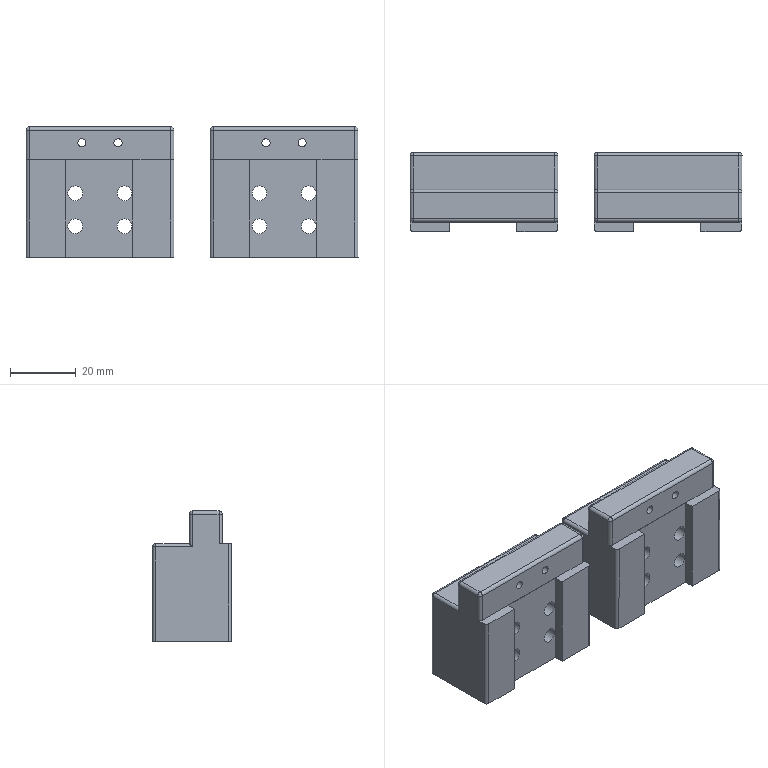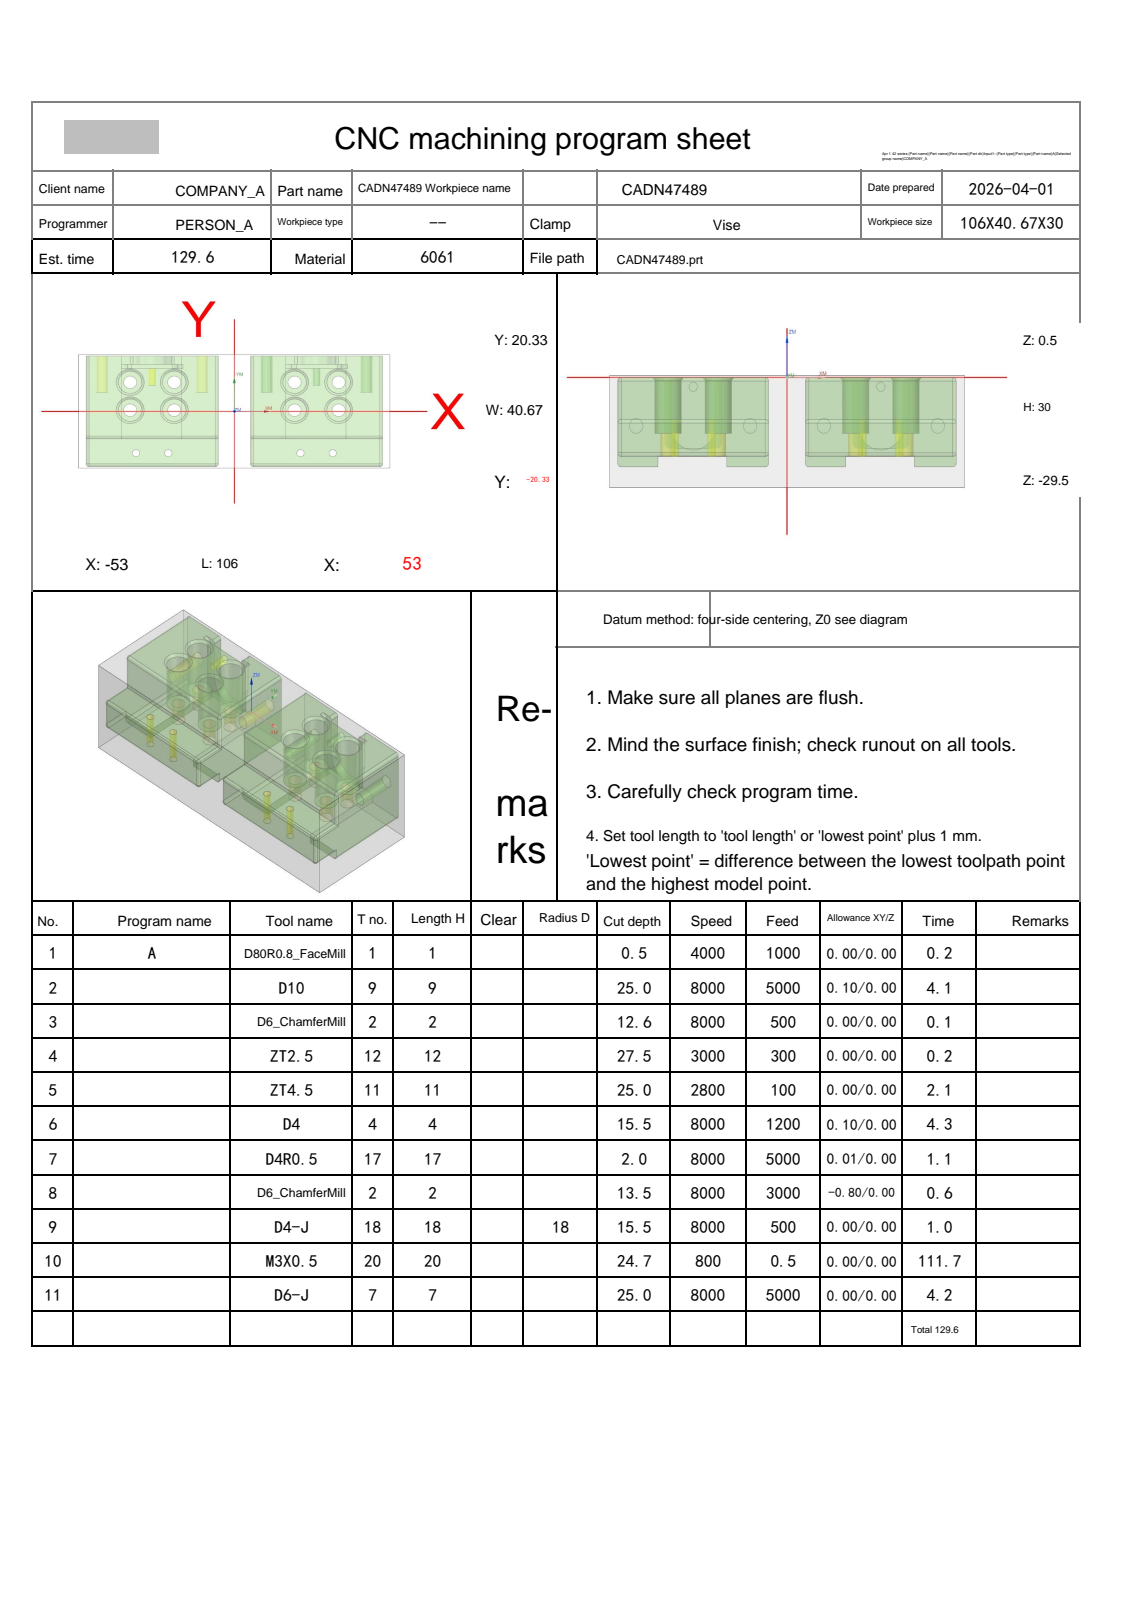NC program | NX | posted by the shop | part box 101.001 x 24.001 x 39.667 mm
Lines 2474 to 3550 of 28944:
N6 T04 M06
(D4  D=4. R=0. H=04 ce=0.10 di=0.00)
G00 G90 G54 X35.5 Y.416 M03 S8000
G43 H04 Z20.
M08
Z.499
G01 X35.513 Y.251 F1200.
X35.555 Y.091
X35.626 Y-.06
X35.721 Y-.196
X35.838 Y-.313
X35.974 Y-.408
X36.124 Y-.478
X36.285 Y-.521
X36.45 Y-.536
X36.615 Y-.521
X36.776 Y-.478
X36.926 Y-.408
X37.062 Y-.313
X37.179 Y-.196
X37.275 Y-.06
X37.345 Y.091
X37.388 Y.251
X37.4 Y.416
X37.386 Y.662 Z.493
X37.338 Y.904 Z.487
X37.26 Y1.138 Z.48
X37.152 Y1.359 Z.474
X37.016 Y1.565 Z.468
X36.855 Y1.752 Z.462
X36.671 Y1.916 Z.456
X36.467 Y2.054 Z.449
X36.247 Y2.166 Z.443
X36.014 Y2.248 Z.437
X35.773 Y2.299 Z.431
X35.528 Y2.318 Z.425
X35.281 Y2.306 Z.419
X35.039 Y2.262 Z.412
X34.804 Y2.186 Z.406
X34.581 Y2.082 Z.4
X34.373 Y1.949 Z.394
X34.185 Y1.79 Z.388
X34.018 Y1.608 Z.381
X33.876 Y1.407 Z.375
X33.762 Y1.188 Z.369
X33.677 Y.957 Z.363
X33.622 Y.717 Z.357
X33.599 Y.471 Z.35
X33.608 Y.225 Z.344
X33.648 Y-.018 Z.338
X33.72 Y-.254 Z.332
X33.822 Y-.479 Z.326
X33.952 Y-.688 Z.319
X34.107 Y-.879 Z.313
X34.287 Y-1.048 Z.307
X34.486 Y-1.193 Z.301
X34.703 Y-1.311 Z.295
X34.933 Y-1.399 Z.288
X35.173 Y-1.457 Z.282
X35.418 Y-1.484 Z.276
X35.664 Y-1.479 Z.27
X35.908 Y-1.441 Z.264
X36.145 Y-1.373 Z.257
X36.371 Y-1.275 Z.251
X36.582 Y-1.148 Z.245
X36.775 Y-.995 Z.239
X36.947 Y-.818 Z.233
X37.095 Y-.62 Z.226
X37.215 Y-.405 Z.22
X37.307 Y-.177 Z.214
X37.369 Y.062 Z.208
X37.399 Y.307 Z.202
X37.397 Y.553 Z.196
X37.364 Y.797 Z.189
X37.299 Y1.035 Z.183
X37.203 Y1.263 Z.177
X37.08 Y1.476 Z.171
X36.929 Y1.671 Z.165
X36.755 Y1.845 Z.158
X36.56 Y1.996 Z.152
X36.347 Y2.12 Z.146
X36.119 Y2.215 Z.14
X35.881 Y2.28 Z.134
X35.637 Y2.313 Z.127
X35.391 Y2.315 Z.121
X35.146 Y2.285 Z.115
X34.907 Y2.224 Z.109
X34.679 Y2.132 Z.103
X34.464 Y2.011 Z.097
X34.266 Y1.864 Z.09
X34.089 Y1.692 Z.084
X33.936 Y1.499 Z.078
X33.809 Y1.287 Z.072
X33.711 Y1.061 Z.066
X33.642 Y.825 Z.059
X33.605 Y.581 Z.053
X33.6 Y.334 Z.047
X33.626 Y.089 Z.041
X33.684 Y-.15 Z.035
X33.773 Y-.38 Z.028
X33.89 Y-.597 Z.022
X34.035 Y-.797 Z.016
X34.204 Y-.976 Z.01
X34.395 Y-1.132 Z.004
X34.605 Y-1.262 Z-.003
X34.829 Y-1.363 Z-.009
X35.065 Y-1.435 Z-.015
X35.308 Y-1.476 Z-.021
X35.555 Y-1.485 Z-.027
X35.8 Y-1.462 Z-.034
X36.04 Y-1.407 Z-.04
X36.272 Y-1.322 Z-.046
X36.49 Y-1.208 Z-.052
X36.692 Y-1.066 Z-.058
X36.873 Y-.899 Z-.065
X37.032 Y-.711 Z-.071
X37.165 Y-.503 Z-.077
X37.27 Y-.28 Z-.083
X37.345 Y-.045 Z-.089
X37.389 Y.197 Z-.096
X37.402 Y.443 Z-.102
X37.382 Y.689 Z-.108
X37.331 Y.93 Z-.114
X37.249 Y1.163 Z-.12
X37.138 Y1.383 Z-.126
X36.999 Y1.587 Z-.133
X36.836 Y1.771 Z-.139
X36.649 Y1.932 Z-.145
X36.443 Y2.068 Z-.151
X36.222 Y2.176 Z-.157
X35.988 Y2.255 Z-.164
X35.746 Y2.302 Z-.17
X35.5 Y2.318 Z-.176
X35.254 Y2.302 Z-.182
X35.013 Y2.255 Z-.188
X34.779 Y2.176 Z-.195
X34.557 Y2.068 Z-.201
X34.352 Y1.933 Z-.207
X34.165 Y1.771 Z-.213
X34.001 Y1.587 Z-.219
X33.862 Y1.384 Z-.226
X33.751 Y1.164 Z-.232
X33.669 Y.931 Z-.238
X33.618 Y.69 Z-.244
X33.598 Y.444 Z-.25
X33.611 Y.198 Z-.257
X33.655 Y-.044 Z-.263
X33.73 Y-.279 Z-.269
X33.835 Y-.502 Z-.275
X33.967 Y-.71 Z-.281
X34.126 Y-.899 Z-.288
X34.308 Y-1.065 Z-.294
X34.509 Y-1.207 Z-.3
X34.728 Y-1.322 Z-.306
X34.959 Y-1.407 Z-.312
X35.199 Y-1.462 Z-.319
X35.445 Y-1.485 Z-.325
X35.691 Y-1.476 Z-.331
X35.934 Y-1.435 Z-.337
X36.17 Y-1.364 Z-.343
X36.395 Y-1.262 Z-.349
X36.604 Y-1.132 Z-.356
X36.795 Y-.976 Z-.362
X36.965 Y-.797 Z-.368
X37.109 Y-.598 Z-.374
X37.227 Y-.381 Z-.38
X37.315 Y-.151 Z-.387
X37.374 Y.089 Z-.393
X37.4 Y.334 Z-.399
X37.395 Y.58 Z-.405
X37.358 Y.824 Z-.411
X37.29 Y1.061 Z-.418
X37.191 Y1.287 Z-.424
X37.064 Y1.498 Z-.43
X36.911 Y1.691 Z-.436
X36.735 Y1.863 Z-.442
X36.537 Y2.011 Z-.448
X36.322 Y2.131 Z-.455
X36.094 Y2.223 Z-.461
X35.855 Y2.285 Z-.467
X35.61 Y2.315 Z-.473
X35.364 Y2.314 Z-.479
X35.119 Y2.28 Z-.486
X34.882 Y2.215 Z-.492
X34.654 Y2.12 Z-.498
X34.441 Y1.996 Z-.504
X34.246 Y1.846 Z-.51
X34.071 Y1.672 Z-.517
X33.921 Y1.476 Z-.523
X33.797 Y1.263 Z-.529
X33.702 Y1.036 Z-.535
X33.637 Y.798 Z-.541
X33.603 Y.554 Z-.548
X33.601 Y.307 Z-.554
X33.631 Y.063 Z-.56
X33.693 Y-.176 Z-.566
X33.784 Y-.405 Z-.572
X33.905 Y-.62 Z-.579
X34.052 Y-.817 Z-.585
X34.224 Y-.994 Z-.591
X34.417 Y-1.147 Z-.597
X34.629 Y-1.274 Z-.603
X34.855 Y-1.373 Z-.61
X35.091 Y-1.441 Z-.616
X35.335 Y-1.478 Z-.622
X35.582 Y-1.484 Z-.628
X35.827 Y-1.457 Z-.634
X36.066 Y-1.399 Z-.641
X36.296 Y-1.311 Z-.647
X36.513 Y-1.193 Z-.653
X36.713 Y-1.049 Z-.659
X36.892 Y-.88 Z-.665
X37.048 Y-.689 Z-.671
X37.178 Y-.479 Z-.678
X37.28 Y-.255 Z-.684
X37.352 Y-.019 Z-.69
X37.392 Y.224 Z-.696
X37.401 Y.471 Z-.702
X37.378 Y.716 Z-.709
X37.324 Y.956 Z-.715
X37.239 Y1.188 Z-.721
X37.124 Y1.406 Z-.727
X36.983 Y1.608 Z-.733
X36.816 Y1.79 Z-.739
X36.627 Y1.948 Z-.746
X36.42 Y2.081 Z-.752
X36.197 Y2.186 Z-.758
X35.962 Y2.261 Z-.764
X35.72 Y2.306 Z-.77
X35.473 Y2.318 Z-.777
X35.228 Y2.299 Z-.783
X34.986 Y2.248 Z-.789
X34.754 Y2.166 Z-.795
X34.534 Y2.055 Z-.801
X34.33 Y1.916 Z-.808
X34.146 Y1.752 Z-.814
X33.985 Y1.566 Z-.82
X33.849 Y1.36 Z-.826
X33.741 Y1.139 Z-.832
X33.662 Y.905 Z-.839
X33.614 Y.663 Z-.845
X33.598 Y.417 Z-.851
X33.614 Y.171 Z-.857
X33.661 Y-.071 Z-.863
X33.74 Y-.304 Z-.87
X33.848 Y-.526 Z-.876
X33.984 Y-.732 Z-.882
X34.145 Y-.918 Z-.888
X34.329 Y-1.082 Z-.894
X34.533 Y-1.221 Z-.901
X34.752 Y-1.333 Z-.907
X34.985 Y-1.415 Z-.913
X35.226 Y-1.466 Z-.919
X35.472 Y-1.485 Z-.925
X35.718 Y-1.473 Z-.932
X35.961 Y-1.429 Z-.938
X36.195 Y-1.354 Z-.944
X36.418 Y-1.249 Z-.95
X36.626 Y-1.116 Z-.956
X36.815 Y-.958 Z-.963
X36.982 Y-.776 Z-.969
X37.123 Y-.575 Z-.975
X37.238 Y-.356 Z-.981
X37.323 Y-.125 Z-.987
X37.378 Y.115 Z-.993
X37.401 Y.361 Z-1.
X37.392 Y.607 Z-1.006
X37.352 Y.85 Z-1.012
X37.28 Y1.086 Z-1.018
X37.179 Y1.311 Z-1.024
X37.049 Y1.52 Z-1.031
X36.893 Y1.711 Z-1.037
X36.714 Y1.881 Z-1.043
X36.514 Y2.025 Z-1.049
X36.298 Y2.143 Z-1.055
X36.068 Y2.232 Z-1.061
X35.828 Y2.29 Z-1.068
X35.583 Y2.317 Z-1.074
X35.337 Y2.311 Z-1.08
X35.093 Y2.274 Z-1.086
X34.856 Y2.206 Z-1.092
X34.63 Y2.108 Z-1.099
X34.419 Y1.981 Z-1.105
X34.225 Y1.828 Z-1.111
X34.053 Y1.651 Z-1.117
X33.906 Y1.454 Z-1.123
X33.785 Y1.239 Z-1.13
X33.693 Y1.01 Z-1.136
X33.632 Y.772 Z-1.142
X33.601 Y.527 Z-1.148
X33.603 Y.28 Z-1.154
X33.636 Y.036 Z-1.161
X33.701 Y-.202 Z-1.167
X33.796 Y-.429 Z-1.173
X33.92 Y-.642 Z-1.179
X34.07 Y-.838 Z-1.185
X34.244 Y-1.012 Z-1.192
X34.44 Y-1.163 Z-1.198
X34.653 Y-1.286 Z-1.204
X34.88 Y-1.382 Z-1.21
X35.118 Y-1.447 Z-1.216
X35.362 Y-1.481 Z-1.223
X35.609 Y-1.482 Z-1.229
X35.853 Y-1.452 Z-1.235
X36.092 Y-1.391 Z-1.241
X36.321 Y-1.299 Z-1.247
X36.536 Y-1.179 Z-1.254
X36.733 Y-1.031 Z-1.26
X36.91 Y-.86 Z-1.266
X37.064 Y-.667 Z-1.272
X37.191 Y-.455 Z-1.278
X37.289 Y-.229 Z-1.285
X37.358 Y.007 Z-1.291
X37.395 Y.251 Z-1.297
X37.4 Y.498 Z-1.303
X37.374 Y.743 Z-1.309
X37.316 Y.982 Z-1.315
X37.227 Y1.212 Z-1.322
X37.11 Y1.429 Z-1.328
X36.966 Y1.629 Z-1.334
X36.796 Y1.808 Z-1.34
X36.606 Y1.964 Z-1.346
X36.396 Y2.094 Z-1.353
X36.172 Y2.196 Z-1.359
X35.936 Y2.268 Z-1.365
X35.693 Y2.309 Z-1.371
X35.446 Y2.318 Z-1.377
X35.201 Y2.295 Z-1.383
X34.96 Y2.24 Z-1.39
X34.729 Y2.155 Z-1.396
X34.511 Y2.041 Z-1.402
X34.309 Y1.899 Z-1.408
X34.127 Y1.733 Z-1.414
X33.968 Y1.544 Z-1.421
X33.835 Y1.337 Z-1.427
X33.73 Y1.114 Z-1.433
X33.655 Y.879 Z-1.439
X33.611 Y.636 Z-1.445
X33.598 Y.39 Z-1.452
X33.618 Y.144 Z-1.458
X33.669 Y-.097 Z-1.464
X33.75 Y-.329 Z-1.47
X33.861 Y-.549 Z-1.476
X34. Y-.753 Z-1.483
X34.164 Y-.937 Z-1.489
X34.35 Y-1.099 Z-1.495
X34.556 Y-1.235 Z-1.501
X34.777 Y-1.343 Z-1.507
X35.011 Y-1.422 Z-1.514
X35.253 Y-1.469 Z-1.52
X35.499 Y-1.486 Z-1.526
X35.745 Y-1.47 Z-1.532
X35.987 Y-1.422 Z-1.538
X36.22 Y-1.344 Z-1.545
X36.442 Y-1.236 Z-1.551
X36.648 Y-1.1 Z-1.557
X36.834 Y-.939 Z-1.563
X36.998 Y-.755 Z-1.569
X37.137 Y-.551 Z-1.576
X37.249 Y-.332 Z-1.582
X37.331 Y-.099 Z-1.588
X37.382 Y.142 Z-1.594
X37.402 Y.388 Z-1.6
X37.39 Y.634 Z-1.606
X37.346 Y.877 Z-1.613
X37.271 Y1.111 Z-1.619
X37.166 Y1.335 Z-1.625
X37.033 Y1.542 Z-1.631
X36.875 Y1.731 Z-1.637
X36.693 Y1.898 Z-1.644
X36.491 Y2.04 Z-1.65
X36.273 Y2.154 Z-1.656
X36.042 Y2.24 Z-1.662
X35.802 Y2.294 Z-1.668
X35.556 Y2.318 Z-1.675
X35.31 Y2.309 Z-1.681
X35.067 Y2.268 Z-1.687
X34.831 Y2.197 Z-1.693
X34.606 Y2.095 Z-1.699
X34.396 Y1.966 Z-1.706
X34.205 Y1.81 Z-1.712
X34.036 Y1.631 Z-1.718
X33.891 Y1.431 Z-1.724
X33.774 Y1.215 Z-1.73
X33.685 Y.985 Z-1.737
X33.627 Y.745 Z-1.743
X33.6 Y.5 Z-1.749
X33.605 Y.254 Z-1.755
X33.642 Y.01 Z-1.761
X33.71 Y-.227 Z-1.768
X33.808 Y-.453 Z-1.774
X33.935 Y-.665 Z-1.78
X34.088 Y-.858 Z-1.786
X34.265 Y-1.03 Z-1.792
X34.462 Y-1.177 Z-1.799
X34.677 Y-1.298 Z-1.805
X34.906 Y-1.39 Z-1.811
X35.144 Y-1.452 Z-1.817
X35.389 Y-1.482 Z-1.823
X35.636 Y-1.481 Z-1.829
X35.88 Y-1.447 Z-1.836
X36.118 Y-1.382 Z-1.842
X36.345 Y-1.287 Z-1.848
X36.558 Y-1.164 Z-1.854
X36.754 Y-1.014 Z-1.86
X36.928 Y-.84 Z-1.867
X37.079 Y-.644 Z-1.873
X37.203 Y-.431 Z-1.879
X37.298 Y-.204 Z-1.885
X37.363 Y.034 Z-1.891
X37.397 Y.278 Z-1.898
X37.399 Y.525 Z-1.904
X37.369 Y.769 Z-1.91
X37.308 Y1.008 Z-1.916
X37.216 Y1.237 Z-1.922
X37.095 Y1.452 Z-1.928
X36.948 Y1.65 Z-1.935
X36.777 Y1.826 Z-1.941
X36.583 Y1.98 Z-1.947
X36.372 Y2.107 Z-1.953
X36.146 Y2.205 Z-1.959
X35.909 Y2.274 Z-1.966
X35.666 Y2.311 Z-1.972
X35.419 Y2.317 Z-1.978
X35.174 Y2.29 Z-1.984
X34.935 Y2.232 Z-1.99
X34.704 Y2.144 Z-1.997
X34.488 Y2.027 Z-2.003
X34.288 Y1.882 Z-2.009
X34.109 Y1.713 Z-2.015
X33.953 Y1.522 Z-2.021
X33.823 Y1.313 Z-2.028
X33.721 Y1.088 Z-2.034
X33.649 Y.853 Z-2.04
X33.608 Y.609 Z-2.046
X33.599 Y.363 Z-2.052
X33.622 Y.118 Z-2.059
X33.676 Y-.123 Z-2.065
X33.761 Y-.354 Z-2.071
X33.875 Y-.573 Z-2.077
X34.017 Y-.774 Z-2.083
X34.183 Y-.956 Z-2.09
X34.372 Y-1.115 Z-2.096
X34.58 Y-1.248 Z-2.102
X34.803 Y-1.353 Z-2.108
X35.037 Y-1.428 Z-2.114
X35.28 Y-1.473 Z-2.121
X35.526 Y-1.485 Z-2.127
X35.772 Y-1.466 Z-2.133
X36.013 Y-1.415 Z-2.139
X36.245 Y-1.333 Z-2.145
X36.465 Y-1.222 Z-2.152
X36.669 Y-1.084 Z-2.158
X36.854 Y-.92 Z-2.164
X37.015 Y-.734 Z-2.17
X37.151 Y-.528 Z-2.176
X37.259 Y-.307 Z-2.182
X37.338 Y-.073 Z-2.189
X37.386 Y.169 Z-2.195
X37.402 Y.415 Z-2.201
X37.386 Y.661 Z-2.207
X37.339 Y.903 Z-2.213
X37.26 Y1.137 Z-2.22
X37.153 Y1.358 Z-2.226
X37.017 Y1.564 Z-2.232
X36.856 Y1.75 Z-2.238
X36.672 Y1.915 Z-2.244
X36.468 Y2.054 Z-2.25
X36.248 Y2.165 Z-2.257
X36.016 Y2.247 Z-2.263
X35.775 Y2.299 Z-2.269
X35.529 Y2.318 Z-2.275
X35.283 Y2.306 Z-2.281
X35.04 Y2.262 Z-2.288
X34.805 Y2.187 Z-2.294
X34.582 Y2.082 Z-2.3
X34.375 Y1.95 Z-2.306
X34.186 Y1.791 Z-2.312
X34.019 Y1.61 Z-2.319
X33.877 Y1.408 Z-2.325
X33.762 Y1.19 Z-2.331
X33.677 Y.959 Z-2.337
X33.622 Y.718 Z-2.343
X33.599 Y.473 Z-2.35
X33.608 Y.227 Z-2.356
X33.648 Y-.017 Z-2.362
X33.72 Y-.252 Z-2.368
X33.821 Y-.477 Z-2.374
X33.951 Y-.687 Z-2.381
X34.106 Y-.878 Z-2.387
X34.286 Y-1.047 Z-2.393
X34.485 Y-1.192 Z-2.399
X34.702 Y-1.31 Z-2.405
X34.932 Y-1.399 Z-2.412
X35.171 Y-1.457 Z-2.418
X35.416 Y-1.484 Z-2.424
X35.663 Y-1.479 Z-2.43
X35.906 Y-1.442 Z-2.436
X36.143 Y-1.373 Z-2.443
X36.369 Y-1.275 Z-2.449
X36.581 Y-1.149 Z-2.455
X36.774 Y-.996 Z-2.461
X36.946 Y-.819 Z-2.467
X37.094 Y-.622 Z-2.473
X37.215 Y-.407 Z-2.48
X37.307 Y-.178 Z-2.486
X37.368 Y.06 Z-2.492
X37.399 Y.305 Z-2.498
X37.397 Y.552 Z-2.504
X37.364 Y.796 Z-2.511
X37.299 Y1.034 Z-2.517
X37.204 Y1.261 Z-2.523
X37.081 Y1.475 Z-2.529
X36.93 Y1.67 Z-2.535
X36.756 Y1.845 Z-2.542
X36.561 Y1.995 Z-2.548
X36.348 Y2.119 Z-2.554
X36.121 Y2.214 Z-2.56
X35.883 Y2.28 Z-2.566
X35.639 Y2.313 Z-2.572
X35.392 Y2.315 Z-2.579
X35.148 Y2.286 Z-2.585
X34.909 Y2.224 Z-2.591
X34.68 Y2.133 Z-2.597
X34.465 Y2.012 Z-2.603
X34.267 Y1.865 Z-2.61
X34.09 Y1.693 Z-2.616
X33.937 Y1.5 Z-2.622
X33.81 Y1.289 Z-2.628
X33.711 Y1.063 Z-2.634
X33.643 Y.826 Z-2.641
X33.605 Y.583 Z-2.647
X33.6 Y.336 Z-2.653
X33.626 Y.091 Z-2.659
X33.684 Y-.149 Z-2.665
X33.772 Y-.379 Z-2.672
X33.89 Y-.596 Z-2.678
X34.034 Y-.795 Z-2.684
X34.203 Y-.975 Z-2.69
X34.394 Y-1.131 Z-2.696
X34.603 Y-1.261 Z-2.703
X34.828 Y-1.363 Z-2.709
X35.064 Y-1.435 Z-2.715
X35.307 Y-1.476 Z-2.721
X35.553 Y-1.485 Z-2.727
X35.798 Y-1.462 Z-2.734
X36.039 Y-1.408 Z-2.74
X36.27 Y-1.323 Z-2.746
X36.489 Y-1.208 Z-2.752
X36.691 Y-1.067 Z-2.758
X36.872 Y-.9 Z-2.765
X37.031 Y-.712 Z-2.771
X37.164 Y-.504 Z-2.777
X37.269 Y-.281 Z-2.783
X37.345 Y-.047 Z-2.789
X37.389 Y.196 Z-2.795
X37.402 Y.442 Z-2.802
X37.383 Y.688 Z-2.808
X37.332 Y.929 Z-2.814
X37.25 Y1.161 Z-2.82
X37.139 Y1.382 Z-2.826
X37. Y1.585 Z-2.833
X36.837 Y1.77 Z-2.839
X36.65 Y1.931 Z-2.845
X36.445 Y2.067 Z-2.851
X36.223 Y2.176 Z-2.857
X35.99 Y2.254 Z-2.864
X35.748 Y2.302 Z-2.87
X35.502 Y2.318 Z-2.876
X35.256 Y2.303 Z-2.882
X35.014 Y2.255 Z-2.888
X34.78 Y2.177 Z-2.894
X34.559 Y2.069 Z-2.901
X34.353 Y1.934 Z-2.907
X34.166 Y1.772 Z-2.913
X34.002 Y1.589 Z-2.919
X33.863 Y1.385 Z-2.925
X33.752 Y1.165 Z-2.932
X33.669 Y.933 Z-2.938
X33.618 Y.692 Z-2.944
X33.598 Y.446 Z-2.95
X33.61 Y.2 Z-2.956
X33.654 Y-.043 Z-2.963
X33.729 Y-.278 Z-2.969
X33.834 Y-.501 Z-2.975
X33.967 Y-.709 Z-2.981
X34.125 Y-.898 Z-2.987
X34.306 Y-1.064 Z-2.994
X34.508 Y-1.206 Z-3.
X34.726 Y-1.321 Z-3.006
X34.957 Y-1.406 Z-3.012
X35.198 Y-1.461 Z-3.018
X35.443 Y-1.485 Z-3.025
X35.69 Y-1.476 Z-3.031
X35.933 Y-1.436 Z-3.037
X36.169 Y-1.364 Z-3.043
X36.393 Y-1.263 Z-3.049
X36.603 Y-1.133 Z-3.056
X36.794 Y-.977 Z-3.062
X36.964 Y-.798 Z-3.068
X37.108 Y-.599 Z-3.074
X37.226 Y-.382 Z-3.08
X37.315 Y-.152 Z-3.087
X37.373 Y.087 Z-3.093
X37.4 Y.332 Z-3.099
X37.395 Y.579 Z-3.105
X37.358 Y.822 Z-3.111
X37.29 Y1.059 Z-3.117
X37.192 Y1.285 Z-3.124
X37.065 Y1.497 Z-3.13
X36.912 Y1.69 Z-3.136
X36.736 Y1.862 Z-3.142
X36.539 Y2.01 Z-3.148
X36.324 Y2.131 Z-3.155
X36.095 Y2.223 Z-3.161
X35.856 Y2.285 Z-3.167
X35.612 Y2.315 Z-3.173
X35.365 Y2.314 Z-3.179
X35.121 Y2.28 Z-3.186
X34.883 Y2.216 Z-3.192
X34.656 Y2.121 Z-3.198
X34.442 Y1.997 Z-3.204
X34.247 Y1.847 Z-3.21
X34.072 Y1.673 Z-3.217
X33.922 Y1.478 Z-3.223
X33.798 Y1.265 Z-3.229
X33.702 Y1.038 Z-3.235
X33.637 Y.8 Z-3.241
X33.603 Y.556 Z-3.248
X33.601 Y.309 Z-3.254
X33.631 Y.064 Z-3.26
X33.692 Y-.174 Z-3.266
X33.784 Y-.403 Z-3.272
X33.904 Y-.618 Z-3.279
X34.051 Y-.816 Z-3.285
X34.223 Y-.993 Z-3.291
X34.416 Y-1.146 Z-3.297
X34.627 Y-1.273 Z-3.303
X34.853 Y-1.372 Z-3.31
X35.09 Y-1.441 Z-3.316
X35.334 Y-1.478 Z-3.322
X35.58 Y-1.484 Z-3.328
X35.825 Y-1.458 Z-3.334
X36.065 Y-1.4 Z-3.34
X36.295 Y-1.311 Z-3.347
X36.512 Y-1.194 Z-3.353
X36.712 Y-1.05 Z-3.359
X36.891 Y-.881 Z-3.365
X37.047 Y-.69 Z-3.371
X37.177 Y-.481 Z-3.378
X37.279 Y-.256 Z-3.384
X37.351 Y-.02 Z-3.39
X37.392 Y.223 Z-3.396
X37.401 Y.469 Z-3.402
X37.379 Y.714 Z-3.409
X37.324 Y.955 Z-3.415
X37.239 Y1.186 Z-3.421
X37.125 Y1.405 Z-3.427
X36.984 Y1.607 Z-3.433
X36.817 Y1.789 Z-3.439
X36.629 Y1.947 Z-3.446
X36.421 Y2.081 Z-3.452
X36.198 Y2.186 Z-3.458
X35.964 Y2.261 Z-3.464
X35.721 Y2.306 Z-3.47
X35.475 Y2.318 Z-3.477
X35.229 Y2.299 Z-3.483
X34.988 Y2.248 Z-3.489
X34.755 Y2.167 Z-3.495
X34.535 Y2.056 Z-3.501
X34.331 Y1.917 Z-3.508
X34.147 Y1.753 Z-3.514
X33.986 Y1.567 Z-3.52
X33.849 Y1.362 Z-3.526
X33.741 Y1.14 Z-3.532
X33.662 Y.907 Z-3.539
X33.614 Y.665 Z-3.545
X33.598 Y.419 Z-3.551
X33.614 Y.173 Z-3.557
X33.661 Y-.069 Z-3.563
X33.739 Y-.303 Z-3.57
X33.847 Y-.524 Z-3.576
X33.983 Y-.73 Z-3.582
X34.144 Y-.917 Z-3.588
X34.328 Y-1.081 Z-3.594
X34.531 Y-1.22 Z-3.601
X34.751 Y-1.332 Z-3.607
X34.983 Y-1.414 Z-3.613
X35.224 Y-1.465 Z-3.619
X35.47 Y-1.485 Z-3.625
X35.716 Y-1.473 Z-3.632
X35.959 Y-1.429 Z-3.638
X36.194 Y-1.354 Z-3.644
X36.417 Y-1.25 Z-3.65
X36.625 Y-1.117 Z-3.656
X36.814 Y-.959 Z-3.662
X36.981 Y-.777 Z-3.669
X37.123 Y-.576 Z-3.675
X37.237 Y-.358 Z-3.681
X37.323 Y-.126 Z-3.687
X37.378 Y.114 Z-3.693
X37.401 Y.359 Z-3.7
X37.393 Y.606 Z-3.706
X37.352 Y.849 Z-3.712
X37.281 Y1.085 Z-3.718
X37.179 Y1.309 Z-3.724
X37.05 Y1.519 Z-3.731
X36.894 Y1.71 Z-3.737
X36.715 Y1.88 Z-3.743
X36.516 Y2.025 Z-3.749
X36.299 Y2.142 Z-3.755
X36.069 Y2.231 Z-3.761
X35.83 Y2.29 Z-3.768
X35.585 Y2.317 Z-3.774
X35.338 Y2.312 Z-3.78
X35.095 Y2.275 Z-3.786
X34.858 Y2.207 Z-3.792
X34.631 Y2.109 Z-3.799
X34.42 Y1.982 Z-3.805
X34.227 Y1.829 Z-3.811
X34.055 Y1.653 Z-3.817
X33.907 Y1.455 Z-3.823
X33.786 Y1.241 Z-3.83
X33.694 Y1.012 Z-3.836
X33.632 Y.773 Z-3.842
X33.601 Y.529 Z-3.848
X33.603 Y.282 Z-3.854
X33.636 Y.038 Z-3.861
X33.701 Y-.2 Z-3.867
X33.796 Y-.428 Z-3.873
X33.919 Y-.641 Z-3.879
X34.069 Y-.836 Z-3.885
X34.243 Y-1.011 Z-3.892
X34.438 Y-1.162 Z-3.898
X34.651 Y-1.286 Z-3.904
X34.879 Y-1.381 Z-3.91
X35.116 Y-1.446 Z-3.916
X35.361 Y-1.48 Z-3.923
X35.607 Y-1.482 Z-3.929
X35.852 Y-1.453 Z-3.935
X36.091 Y-1.392 Z-3.941
X36.319 Y-1.3 Z-3.947
X36.535 Y-1.18 Z-3.954
X36.732 Y-1.032 Z-3.96
X36.909 Y-.861 Z-3.966
X37.063 Y-.668 Z-3.972
X37.19 Y-.457 Z-3.978
X37.289 Y-.231 Z-3.984
X37.357 Y.006 Z-3.991
X37.395 Y.25 Z-3.997
X37.4 Y.496 Z-4.003
X37.374 Y.741 Z-4.009
X37.316 Y.981 Z-4.015
X37.228 Y1.211 Z-4.022
X37.111 Y1.428 Z-4.028
X36.967 Y1.628 Z-4.034
X36.798 Y1.807 Z-4.04
X36.607 Y1.963 Z-4.046
X36.397 Y2.093 Z-4.053
X36.173 Y2.195 Z-4.059
X35.937 Y2.268 Z-4.065
X35.694 Y2.309 Z-4.071
X35.448 Y2.318 Z-4.077
X35.202 Y2.295 Z-4.083
X34.962 Y2.241 Z-4.09
X34.731 Y2.156 Z-4.096
X34.512 Y2.042 Z-4.102
X34.31 Y1.9 Z-4.108
X34.128 Y1.734 Z-4.114
X33.969 Y1.546 Z-4.121
X33.836 Y1.338 Z-4.127
X33.731 Y1.115 Z-4.133
X33.655 Y.88 Z-4.139
X33.611 Y.638 Z-4.145
X33.598 Y.392 Z-4.152
X33.617 Y.146 Z-4.158
X33.668 Y-.095 Z-4.164
X33.75 Y-.328 Z-4.17
X33.861 Y-.548 Z-4.176
X33.999 Y-.752 Z-4.183
X34.163 Y-.936 Z-4.189
X34.349 Y-1.098 Z-4.195
X34.555 Y-1.234 Z-4.201
X34.776 Y-1.342 Z-4.207
X35.009 Y-1.421 Z-4.214
X35.251 Y-1.469 Z-4.22
X35.497 Y-1.485 Z-4.226
X35.743 Y-1.47 Z-4.232
X35.985 Y-1.423 Z-4.238
X36.219 Y-1.344 Z-4.245
X36.441 Y-1.237 Z-4.251
X36.647 Y-1.101 Z-4.257
X36.833 Y-.94 Z-4.263
X36.997 Y-.756 Z-4.269
X37.137 Y-.553 Z-4.276
X37.248 Y-.333 Z-4.282
X37.33 Y-.1 Z-4.288
X37.382 Y.141 Z-4.294
X37.402 Y.386 Z-4.3
X37.39 Y.633 Z-4.306
X37.346 Y.875 Z-4.313
X37.271 Y1.11 Z-4.319
X37.167 Y1.333 Z-4.325
X37.034 Y1.541 Z-4.331
X36.876 Y1.73 Z-4.337
X36.694 Y1.897 Z-4.344
X36.493 Y2.039 Z-4.35
X36.275 Y2.154 Z-4.356
X36.043 Y2.239 Z-4.362
X35.803 Y2.294 Z-4.368
X35.558 Y2.318 Z-4.375
X35.311 Y2.309 Z-4.381
X35.068 Y2.269 Z-4.387
X34.832 Y2.197 Z-4.393
X34.607 Y2.096 Z-4.399
X34.398 Y1.967 Z-4.405
X34.207 Y1.811 Z-4.412
X34.037 Y1.632 Z-4.418
X33.892 Y1.433 Z-4.424
X33.774 Y1.216 Z-4.43
X33.685 Y.986 Z-4.436
X33.627 Y.747 Z-4.443
X33.6 Y.502 Z-4.449
X33.605 Y.255 Z-4.455
X33.642 Y.011 Z-4.461
X33.71 Y-.226 Z-4.467
X33.808 Y-.452 Z-4.474
X33.934 Y-.663 Z-4.48
X34.087 Y-.857 Z-4.486
X34.264 Y-1.029 Z-4.492
X34.461 Y-1.177 Z-4.498
X34.676 Y-1.298 Z-4.505
X34.904 Y-1.39 Z-4.511
X35.143 Y-1.452 Z-4.517
X35.387 Y-1.482 Z-4.523
X35.634 Y-1.481 Z-4.529
X35.878 Y-1.447 Z-4.536
X36.116 Y-1.383 Z-4.542
X36.344 Y-1.288 Z-4.548
X36.557 Y-1.165 Z-4.554
X36.753 Y-1.015 Z-4.56
X36.927 Y-.841 Z-4.567
X37.078 Y-.645 Z-4.573
X37.202 Y-.432 Z-4.579
X37.298 Y-.205 Z-4.585
X37.363 Y.032 Z-4.591
X37.397 Y.277 Z-4.598
X37.399 Y.523 Z-4.604
X37.369 Y.768 Z-4.61
X37.308 Y1.007 Z-4.616
X37.217 Y1.236 Z-4.622
X37.096 Y1.451 Z-4.628
X36.949 Y1.648 Z-4.635
X36.778 Y1.826 Z-4.641
X36.585 Y1.979 Z-4.647
X36.374 Y2.106 Z-4.653
X36.148 Y2.205 Z-4.659
X35.911 Y2.274 Z-4.666
X35.667 Y2.311 Z-4.672
X35.421 Y2.317 Z-4.678
X35.176 Y2.291 Z-4.684
X34.936 Y2.233 Z-4.69
X34.706 Y2.145 Z-4.697
X34.489 Y2.028 Z-4.703
X34.289 Y1.883 Z-4.709
X34.11 Y1.714 Z-4.715
X33.953 Y1.524 Z-4.721
X33.823 Y1.314 Z-4.728
X33.721 Y1.09 Z-4.734
X33.649 Y.854 Z-4.74
X33.608 Y.611 Z-4.746
X33.599 Y.365 Z-4.752
X33.621 Y.119 Z-4.759
X33.676 Y-.121 Z-4.765
X33.76 Y-.353 Z-4.771
X33.875 Y-.571 Z-4.777
X34.016 Y-.773 Z-4.783
X34.182 Y-.955 Z-4.79
X34.371 Y-1.114 Z-4.796
X34.578 Y-1.247 Z-4.802
X34.801 Y-1.352 Z-4.808
X35.036 Y-1.428 Z-4.814
X35.278 Y-1.472 Z-4.821
X35.524 Y-1.485 Z-4.827
X35.77 Y-1.466 Z-4.833
X36.011 Y-1.415 Z-4.839
X36.244 Y-1.334 Z-4.845
X36.464 Y-1.223 Z-4.851
X36.668 Y-1.085 Z-4.858
X36.852 Y-.921 Z-4.864
X37.014 Y-.735 Z-4.87
X37.15 Y-.529 Z-4.876
X37.259 Y-.308 Z-4.882
X37.338 Y-.074 Z-4.889
X37.386 Y.167 Z-4.895
X37.402 Y.413 Z-4.901
X37.386 Y.659 Z-4.907
X37.339 Y.901 Z-4.913
X37.261 Y1.135 Z-4.92
X37.153 Y1.357 Z-4.926
X37.018 Y1.563 Z-4.932
X36.857 Y1.749 Z-4.938
X36.673 Y1.914 Z-4.944
X36.47 Y2.053 Z-4.95
X36.25 Y2.165 Z-4.957
X36.017 Y2.247 Z-4.963
X35.776 Y2.298 Z-4.969
X35.531 Y2.318 Z-4.975
X35.284 Y2.306 Z-4.981
X35.042 Y2.263 Z-4.988
X34.807 Y2.188 Z-4.994
X34.584 Y2.083 Z-5.
X34.376 Y1.951 Z-5.006
X34.187 Y1.792 Z-5.012
X34.02 Y1.611 Z-5.019
X33.878 Y1.41 Z-5.025
X33.763 Y1.191 Z-5.031
X33.677 Y.96 Z-5.037
X33.622 Y.72 Z-5.043
X33.599 Y.475 Z-5.05
X33.607 Y.228 Z-5.056
X33.648 Y-.015 Z-5.062
X33.719 Y-.251 Z-5.068
X33.82 Y-.476 Z-5.074
X33.95 Y-.685 Z-5.081
X34.105 Y-.877 Z-5.087
X34.284 Y-1.046 Z-5.093
X34.484 Y-1.191 Z-5.099
X34.7 Y-1.309 Z-5.105
X34.93 Y-1.398 Z-5.112
X35.169 Y-1.457 Z-5.118
X35.415 Y-1.484 Z-5.124
X35.661 Y-1.479 Z-5.13
X35.905 Y-1.442 Z-5.136
X36.142 Y-1.374 Z-5.143
X36.368 Y-1.276 Z-5.149
X36.579 Y-1.149 Z-5.155
X36.773 Y-.997 Z-5.161
X36.945 Y-.82 Z-5.167
X37.093 Y-.623 Z-5.173
X37.214 Y-.408 Z-5.18
X37.306 Y-.18 Z-5.186
X37.368 Y.059 Z-5.192
X37.399 Y.304 Z-5.198
X37.397 Y.55 Z-5.204
X37.364 Y.794 Z-5.211
X37.3 Y1.032 Z-5.217
X37.205 Y1.26 Z-5.223
X37.081 Y1.473 Z-5.229
X36.932 Y1.669 Z-5.235
X36.758 Y1.844 Z-5.241
X36.562 Y1.994 Z-5.248
X36.349 Y2.118 Z-5.254
X36.122 Y2.214 Z-5.26
X35.884 Y2.279 Z-5.266
X35.64 Y2.313 Z-5.272
X35.394 Y2.316 Z-5.279
X35.149 Y2.286 Z-5.285
X34.91 Y2.225 Z-5.291
X34.681 Y2.133 Z-5.297
X34.466 Y2.013 Z-5.303
X34.268 Y1.866 Z-5.31
X34.091 Y1.695 Z-5.316
X33.938 Y1.502 Z-5.322
X33.811 Y1.29 Z-5.328
X33.712 Y1.065 Z-5.334
X33.643 Y.828 Z-5.341
X33.605 Y.584 Z-5.347
X33.6 Y.338 Z-5.353
X33.626 Y.093 Z-5.359
X33.683 Y-.147 Z-5.365
X33.772 Y-.377 Z-5.372
X33.889 Y-.594 Z-5.378
X34.033 Y-.794 Z-5.384
X34.202 Y-.974 Z-5.39
X34.393 Y-1.13 Z-5.396
X34.602 Y-1.26 Z-5.403
X34.826 Y-1.362 Z-5.409
X35.062 Y-1.434 Z-5.415
X35.305 Y-1.475 Z-5.421
X35.551 Y-1.485 Z-5.427
X35.797 Y-1.462 Z-5.434
X36.037 Y-1.408 Z-5.44
X36.269 Y-1.323 Z-5.446
X36.487 Y-1.209 Z-5.452
X36.689 Y-1.068 Z-5.458
X36.871 Y-.902 Z-5.465
X37.03 Y-.713 Z-5.471
X37.163 Y-.506 Z-5.477
X37.269 Y-.283 Z-5.483
X37.344 Y-.048 Z-5.489
X37.389 Y.194 Z-5.495
X37.402 Y.44 Z-5.502
X37.383 Y.686 Z-5.508
X37.332 Y.927 Z-5.514
X37.251 Y1.16 Z-5.52
X37.14 Y1.38 Z-5.526
X37.001 Y1.584 Z-5.533
X36.838 Y1.769 Z-5.539
X36.652 Y1.93 Z-5.545
X36.446 Y2.067 Z-5.551
X36.225 Y2.175 Z-5.557
X35.991 Y2.254 Z-5.563
X35.75 Y2.302 Z-5.57
X35.504 Y2.319 Z-5.576
X35.258 Y2.303 Z-5.582
X35.016 Y2.256 Z-5.588
X34.782 Y2.178 Z-5.594
X34.56 Y2.07 Z-5.601
X34.354 Y1.935 Z-5.607
X34.167 Y1.774 Z-5.613
X34.003 Y1.59 Z-5.619
X33.864 Y1.386 Z-5.625
X33.752 Y1.167 Z-5.632
X33.67 Y.934 Z-5.638
X33.618 Y.693 Z-5.644
X33.598 Y.448 Z-5.65
X33.61 Y.201 Z-5.656
X33.654 Y-.041 Z-5.663
X33.729 Y-.276 Z-5.669
X33.833 Y-.499 Z-5.675
X33.966 Y-.707 Z-5.681
X34.124 Y-.896 Z-5.687
X34.305 Y-1.063 Z-5.694
X34.507 Y-1.205 Z-5.7
X34.725 Y-1.32 Z-5.706
X34.956 Y-1.406 Z-5.712
X35.196 Y-1.461 Z-5.718
X35.442 Y-1.485 Z-5.725
X35.688 Y-1.476 Z-5.731
X35.931 Y-1.436 Z-5.737
X36.167 Y-1.365 Z-5.743
X36.392 Y-1.263 Z-5.749
X36.602 Y-1.134 Z-5.756
X36.793 Y-.978 Z-5.762
X36.962 Y-.799 Z-5.768
X37.107 Y-.6 Z-5.774
X37.225 Y-.384 Z-5.78
X37.314 Y-.154 Z-5.787
X37.373 Y.086 Z-5.793
X37.4 Y.331 Z-5.799
X37.395 Y.577 Z-5.805
X37.359 Y.821 Z-5.811
X37.291 Y1.058 Z-5.817
X37.193 Y1.284 Z-5.824
X37.066 Y1.496 Z-5.83
X36.914 Y1.689 Z-5.836
X36.737 Y1.861 Z-5.842
X36.54 Y2.009 Z-5.848
X36.325 Y2.13 Z-5.855
X36.097 Y2.223 Z-5.861
X35.858 Y2.285 Z-5.867
X35.613 Y2.315 Z-5.873
X35.367 Y2.314 Z-5.879
X35.123 Y2.281 Z-5.885
X34.885 Y2.216 Z-5.892
X34.657 Y2.122 Z-5.898
X34.444 Y1.998 Z-5.904
X34.248 Y1.848 Z-5.91
X34.073 Y1.674 Z-5.916
X33.923 Y1.479 Z-5.923
X33.798 Y1.266 Z-5.929
X33.703 Y1.039 Z-5.935
X33.637 Y.801 Z-5.941
X33.603 Y.557 Z-5.947
X33.601 Y.311 Z-5.954
X33.631 Y.066 Z-5.96
X33.692 Y-.173 Z-5.966
X33.783 Y-.402 Z-5.972
X33.903 Y-.617 Z-5.978
X34.05 Y-.815 Z-5.985
X34.222 Y-.992 Z-5.991
X34.415 Y-1.145 Z-5.997
X34.626 Y-1.273 Z-6.003
X34.852 Y-1.371 Z-6.009
X35.088 Y-1.44 Z-6.016
X35.332 Y-1.478 Z-6.022